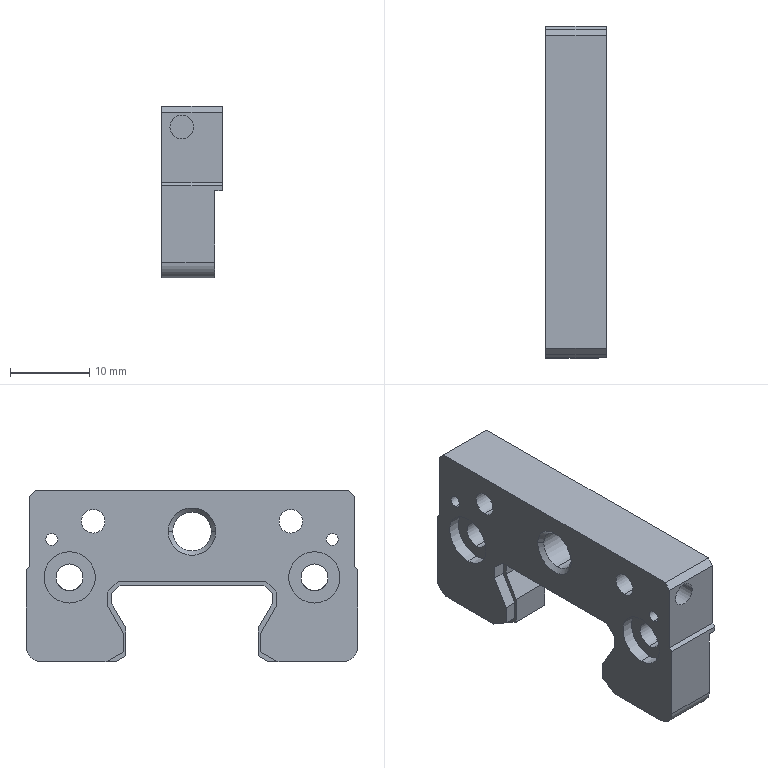Part | NX | 1 solid | 72 faces | box 7.7 x 42 x 21.75 mm | volume 4750 mm3 | plane 44 | cylinder 24 | cone 4 | commonest cylinder face diameters 3 x8 1.51 x4 3.4 x4 6.5 x4 4 x2 4.917 x2